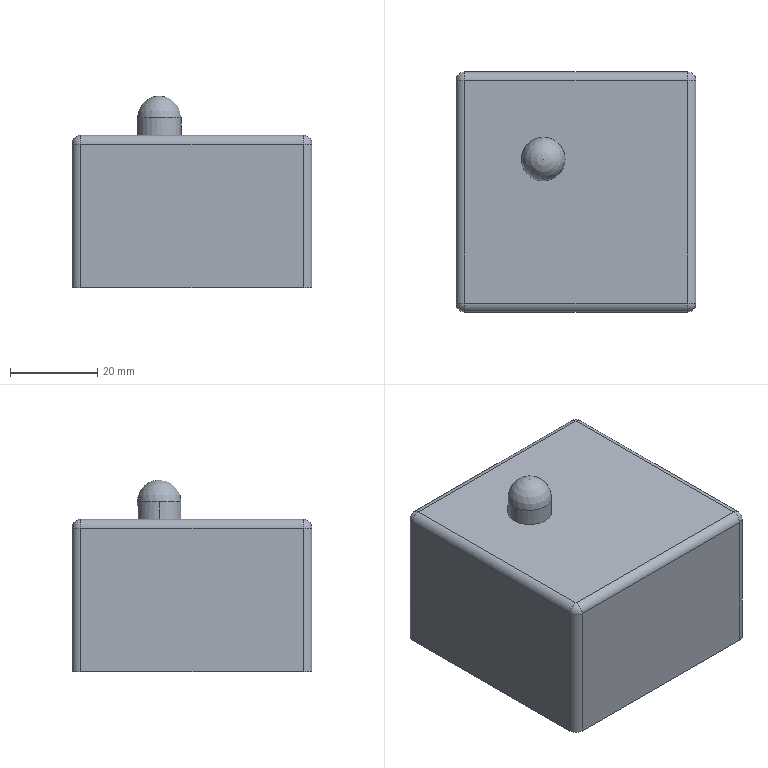Part | SolidWorks | features BaseBody 1 | 1 solid | 21 faces | box 55 x 55 x 44 mm | volume 106147 mm3 | cylinder 10 | plane 6 | sphere 5 | commonest cylinder face diameters 4 x8 10 x2
STEP:
#1=CARTESIAN_POINT('',(25.,-20.,39.));
#2=VERTEX_POINT('',#1);
#3=CARTESIAN_POINT('',(15.,-20.,39.));
#4=VERTEX_POINT('',#3);
#5=CARTESIAN_POINT('',(20.,-20.,39.));
#6=DIRECTION('',(0.,0.,1.));
#7=DIRECTION('',(1.,0.,0.));
#8=AXIS2_PLACEMENT_3D('',#5,#6,#7);
#9=CIRCLE('',#8,5.);
#10=EDGE_CURVE('',#2,#4,#9,.T.);
#11=ORIENTED_EDGE('',*,*,#10,.F.);
#12=CARTESIAN_POINT('',(25.,-20.,35.));
#13=VERTEX_POINT('',#12);
#14=CARTESIAN_POINT('',(25.,-20.,39.));
#15=DIRECTION('',(0.,0.,-1.));
#16=VECTOR('',#15,1000.);
#17=LINE('',#14,#16);
#18=EDGE_CURVE('',#2,#13,#17,.T.);
#19=ORIENTED_EDGE('',*,*,#18,.T.);
#20=CARTESIAN_POINT('',(15.,-20.,35.));
#21=VERTEX_POINT('',#20);
#22=CARTESIAN_POINT('',(20.,-20.,35.));
#23=DIRECTION('',(0.,0.,1.));
#24=DIRECTION('',(1.,0.,0.));
#25=AXIS2_PLACEMENT_3D('',#22,#23,#24);
#26=CIRCLE('',#25,5.);
#27=EDGE_CURVE('',#13,#21,#26,.T.);
#28=ORIENTED_EDGE('',*,*,#27,.T.);
#29=CARTESIAN_POINT('',(15.,-20.,39.));
#30=DIRECTION('',(0.,0.,-1.));
#31=VECTOR('',#30,1000.);
#32=LINE('',#29,#31);
#33=EDGE_CURVE('',#4,#21,#32,.T.);
#34=ORIENTED_EDGE('',*,*,#33,.F.);
#35=EDGE_LOOP('',(#11,#19,#28,#34));
#36=FACE_OUTER_BOUND('',#35,.T.);
#37=CARTESIAN_POINT('',(20.,-20.,39.));
#38=DIRECTION('',(0.,0.,-1.));
#39=DIRECTION('',(-1.,0.,0.));
#40=AXIS2_PLACEMENT_3D('',#37,#38,#39);
#41=CYLINDRICAL_SURFACE('',#40,5.);
#42=ADVANCED_FACE('',(#36),#41,.T.);
#43=CARTESIAN_POINT('',(0.,-2.,0.));
#44=VERTEX_POINT('',#43);
#45=CARTESIAN_POINT('',(0.,-53.,0.));
#46=VERTEX_POINT('',#45);
#47=CARTESIAN_POINT('',(0.,0.,0.));
#48=DIRECTION('',(0.,-1.,0.));
#49=VECTOR('',#48,1000.);
#50=LINE('',#47,#49);
#51=EDGE_CURVE('',#44,#46,#50,.T.);
#52=ORIENTED_EDGE('',*,*,#51,.T.);
#53=CARTESIAN_POINT('',(0.,-53.,33.));
#54=VERTEX_POINT('',#53);
#55=CARTESIAN_POINT('',(0.,-53.,35.));
#56=DIRECTION('',(0.,0.,1.));
#57=VECTOR('',#56,1000.);
#58=LINE('',#55,#57);
#59=EDGE_CURVE('',#46,#54,#58,.T.);
#60=ORIENTED_EDGE('',*,*,#59,.T.);
#61=CARTESIAN_POINT('',(0.,-2.,33.));
#62=VERTEX_POINT('',#61);
#63=CARTESIAN_POINT('',(0.,0.,33.));
#64=DIRECTION('',(0.,1.,0.));
#65=VECTOR('',#64,1000.);
#66=LINE('',#63,#65);
#67=EDGE_CURVE('',#54,#62,#66,.T.);
#68=ORIENTED_EDGE('',*,*,#67,.T.);
#69=CARTESIAN_POINT('',(0.,-2.,35.));
#70=DIRECTION('',(0.,0.,-1.));
#71=VECTOR('',#70,1000.);
#72=LINE('',#69,#71);
#73=EDGE_CURVE('',#62,#44,#72,.T.);
#74=ORIENTED_EDGE('',*,*,#73,.T.);
#75=EDGE_LOOP('',(#52,#60,#68,#74));
#76=FACE_OUTER_BOUND('',#75,.T.);
#77=CARTESIAN_POINT('',(0.,0.,35.));
#78=DIRECTION('',(1.,0.,0.));
#79=DIRECTION('',(0.,1.,0.));
#80=AXIS2_PLACEMENT_3D('',#77,#78,#79);
#81=PLANE('',#80);
#82=ADVANCED_FACE('',(#76),#81,.F.);
#83=CARTESIAN_POINT('',(53.,-55.,33.));
#84=VERTEX_POINT('',#83);
#85=CARTESIAN_POINT('',(2.,-55.,33.));
#86=VERTEX_POINT('',#85);
#87=CARTESIAN_POINT('',(0.,-55.,33.));
#88=DIRECTION('',(-1.,0.,0.));
#89=VECTOR('',#88,1000.);
#90=LINE('',#87,#89);
#91=EDGE_CURVE('',#84,#86,#90,.T.);
#92=ORIENTED_EDGE('',*,*,#91,.T.);
#93=CARTESIAN_POINT('',(2.,-55.,0.));
#94=VERTEX_POINT('',#93);
#95=CARTESIAN_POINT('',(2.,-55.,35.));
#96=DIRECTION('',(0.,0.,-1.));
#97=VECTOR('',#96,1000.);
#98=LINE('',#95,#97);
#99=EDGE_CURVE('',#86,#94,#98,.T.);
#100=ORIENTED_EDGE('',*,*,#99,.T.);
#101=CARTESIAN_POINT('',(53.,-55.,0.));
#102=VERTEX_POINT('',#101);
#103=CARTESIAN_POINT('',(0.,-55.,0.));
#104=DIRECTION('',(1.,0.,0.));
#105=VECTOR('',#104,1000.);
#106=LINE('',#103,#105);
#107=EDGE_CURVE('',#94,#102,#106,.T.);
#108=ORIENTED_EDGE('',*,*,#107,.T.);
#109=CARTESIAN_POINT('',(53.,-55.,35.));
#110=DIRECTION('',(0.,0.,1.));
#111=VECTOR('',#110,1000.);
#112=LINE('',#109,#111);
#113=EDGE_CURVE('',#102,#84,#112,.T.);
#114=ORIENTED_EDGE('',*,*,#113,.T.);
#115=EDGE_LOOP('',(#92,#100,#108,#114));
#116=FACE_OUTER_BOUND('',#115,.T.);
#117=CARTESIAN_POINT('',(0.,-55.,35.));
#118=DIRECTION('',(0.,1.,0.));
#119=DIRECTION('',(0.,0.,1.));
#120=AXIS2_PLACEMENT_3D('',#117,#118,#119);
#121=PLANE('',#120);
#122=ADVANCED_FACE('',(#116),#121,.F.);
#123=CARTESIAN_POINT('',(55.,-53.,0.));
#124=VERTEX_POINT('',#123);
#125=CARTESIAN_POINT('',(55.,-2.,0.));
#126=VERTEX_POINT('',#125);
#127=CARTESIAN_POINT('',(55.,0.,0.));
#128=DIRECTION('',(0.,1.,0.));
#129=VECTOR('',#128,1000.);
#130=LINE('',#127,#129);
#131=EDGE_CURVE('',#124,#126,#130,.T.);
#132=ORIENTED_EDGE('',*,*,#131,.T.);
#133=CARTESIAN_POINT('',(55.,-2.,33.));
#134=VERTEX_POINT('',#133);
#135=CARTESIAN_POINT('',(55.,-2.,35.));
#136=DIRECTION('',(0.,0.,1.));
#137=VECTOR('',#136,1000.);
#138=LINE('',#135,#137);
#139=EDGE_CURVE('',#126,#134,#138,.T.);
#140=ORIENTED_EDGE('',*,*,#139,.T.);
#141=CARTESIAN_POINT('',(55.,-53.,33.));
#142=VERTEX_POINT('',#141);
#143=CARTESIAN_POINT('',(55.,-55.,33.));
#144=DIRECTION('',(0.,-1.,0.));
#145=VECTOR('',#144,1000.);
#146=LINE('',#143,#145);
#147=EDGE_CURVE('',#134,#142,#146,.T.);
#148=ORIENTED_EDGE('',*,*,#147,.T.);
#149=CARTESIAN_POINT('',(55.,-53.,35.));
#150=DIRECTION('',(0.,0.,-1.));
#151=VECTOR('',#150,1000.);
#152=LINE('',#149,#151);
#153=EDGE_CURVE('',#142,#124,#152,.T.);
#154=ORIENTED_EDGE('',*,*,#153,.T.);
#155=EDGE_LOOP('',(#132,#140,#148,#154));
#156=FACE_OUTER_BOUND('',#155,.T.);
#157=CARTESIAN_POINT('',(55.,0.,35.));
#158=DIRECTION('',(-1.,0.,0.));
#159=DIRECTION('',(0.,0.,1.));
#160=AXIS2_PLACEMENT_3D('',#157,#158,#159);
#161=PLANE('',#160);
#162=ADVANCED_FACE('',(#156),#161,.F.);
#163=CARTESIAN_POINT('',(53.,0.,0.));
#164=VERTEX_POINT('',#163);
#165=CARTESIAN_POINT('',(2.,0.,0.));
#166=VERTEX_POINT('',#165);
#167=CARTESIAN_POINT('',(0.,0.,0.));
#168=DIRECTION('',(-1.,0.,0.));
#169=VECTOR('',#168,1000.);
#170=LINE('',#167,#169);
#171=EDGE_CURVE('',#164,#166,#170,.T.);
#172=ORIENTED_EDGE('',*,*,#171,.T.);
#173=CARTESIAN_POINT('',(2.,0.,33.));
#174=VERTEX_POINT('',#173);
#175=CARTESIAN_POINT('',(2.,0.,35.));
#176=DIRECTION('',(0.,0.,1.));
#177=VECTOR('',#176,1000.);
#178=LINE('',#175,#177);
#179=EDGE_CURVE('',#166,#174,#178,.T.);
#180=ORIENTED_EDGE('',*,*,#179,.T.);
#181=CARTESIAN_POINT('',(53.,0.,33.));
#182=VERTEX_POINT('',#181);
#183=CARTESIAN_POINT('',(55.,0.,33.));
#184=DIRECTION('',(1.,0.,0.));
#185=VECTOR('',#184,1000.);
#186=LINE('',#183,#185);
#187=EDGE_CURVE('',#174,#182,#186,.T.);
#188=ORIENTED_EDGE('',*,*,#187,.T.);
#189=CARTESIAN_POINT('',(53.,0.,35.));
#190=DIRECTION('',(0.,0.,-1.));
#191=VECTOR('',#190,1000.);
#192=LINE('',#189,#191);
#193=EDGE_CURVE('',#182,#164,#192,.T.);
#194=ORIENTED_EDGE('',*,*,#193,.T.);
#195=EDGE_LOOP('',(#172,#180,#188,#194));
#196=FACE_OUTER_BOUND('',#195,.T.);
#197=CARTESIAN_POINT('',(0.,0.,35.));
#198=DIRECTION('',(0.,-1.,0.));
#199=DIRECTION('',(0.,0.,-1.));
#200=AXIS2_PLACEMENT_3D('',#197,#198,#199);
#201=PLANE('',#200);
#202=ADVANCED_FACE('',(#196),#201,.F.);
#203=CARTESIAN_POINT('',(53.,-53.,35.));
#204=VERTEX_POINT('',#203);
#205=CARTESIAN_POINT('',(53.,-2.,35.));
#206=VERTEX_POINT('',#205);
#207=CARTESIAN_POINT('',(53.,0.,35.));
#208=DIRECTION('',(0.,1.,0.));
#209=VECTOR('',#208,1000.);
#210=LINE('',#207,#209);
#211=EDGE_CURVE('',#204,#206,#210,.T.);
#212=ORIENTED_EDGE('',*,*,#211,.T.);
#213=CARTESIAN_POINT('',(2.,-2.,35.));
#214=VERTEX_POINT('',#213);
#215=CARTESIAN_POINT('',(0.,-2.,35.));
#216=DIRECTION('',(-1.,0.,0.));
#217=VECTOR('',#216,1000.);
#218=LINE('',#215,#217);
#219=EDGE_CURVE('',#206,#214,#218,.T.);
#220=ORIENTED_EDGE('',*,*,#219,.T.);
#221=CARTESIAN_POINT('',(2.,-53.,35.));
#222=VERTEX_POINT('',#221);
#223=CARTESIAN_POINT('',(2.,-55.,35.));
#224=DIRECTION('',(0.,-1.,0.));
#225=VECTOR('',#224,1000.);
#226=LINE('',#223,#225);
#227=EDGE_CURVE('',#214,#222,#226,.T.);
#228=ORIENTED_EDGE('',*,*,#227,.T.);
#229=CARTESIAN_POINT('',(55.,-53.,35.));
#230=DIRECTION('',(1.,0.,0.));
#231=VECTOR('',#230,1000.);
#232=LINE('',#229,#231);
#233=EDGE_CURVE('',#222,#204,#232,.T.);
#234=ORIENTED_EDGE('',*,*,#233,.T.);
#235=EDGE_LOOP('',(#212,#220,#228,#234));
#236=FACE_OUTER_BOUND('',#235,.T.);
#237=CARTESIAN_POINT('',(20.,-20.,35.));
#238=DIRECTION('',(0.,0.,1.));
#239=DIRECTION('',(1.,0.,0.));
#240=AXIS2_PLACEMENT_3D('',#237,#238,#239);
#241=CIRCLE('',#240,5.);
#242=EDGE_CURVE('',#21,#13,#241,.T.);
#243=ORIENTED_EDGE('',*,*,#242,.F.);
#244=ORIENTED_EDGE('',*,*,#27,.F.);
#245=EDGE_LOOP('',(#243,#244));
#246=FACE_BOUND('',#245,.T.);
#247=CARTESIAN_POINT('',(0.,0.,35.));
#248=DIRECTION('',(0.,0.,1.));
#249=DIRECTION('',(1.,0.,0.));
#250=AXIS2_PLACEMENT_3D('',#247,#248,#249);
#251=PLANE('',#250);
#252=ADVANCED_FACE('',(#236,#246),#251,.T.);
#253=ORIENTED_EDGE('',*,*,#107,.F.);
#254=CARTESIAN_POINT('',(2.,-53.,0.));
#255=DIRECTION('',(0.,0.,-1.));
#256=DIRECTION('',(1.,0.,0.));
#257=AXIS2_PLACEMENT_3D('',#254,#255,#256);
#258=CIRCLE('',#257,2.);
#259=EDGE_CURVE('',#94,#46,#258,.T.);
#260=ORIENTED_EDGE('',*,*,#259,.T.);
#261=ORIENTED_EDGE('',*,*,#51,.F.);
#262=CARTESIAN_POINT('',(2.,-2.,0.));
#263=DIRECTION('',(0.,0.,-1.));
#264=DIRECTION('',(1.,0.,0.));
#265=AXIS2_PLACEMENT_3D('',#262,#263,#264);
#266=CIRCLE('',#265,2.);
#267=EDGE_CURVE('',#44,#166,#266,.T.);
#268=ORIENTED_EDGE('',*,*,#267,.T.);
#269=ORIENTED_EDGE('',*,*,#171,.F.);
#270=CARTESIAN_POINT('',(53.,-2.,0.));
#271=DIRECTION('',(0.,0.,-1.));
#272=DIRECTION('',(1.,0.,0.));
#273=AXIS2_PLACEMENT_3D('',#270,#271,#272);
#274=CIRCLE('',#273,2.);
#275=EDGE_CURVE('',#164,#126,#274,.T.);
#276=ORIENTED_EDGE('',*,*,#275,.T.);
#277=ORIENTED_EDGE('',*,*,#131,.F.);
#278=CARTESIAN_POINT('',(53.,-53.,0.));
#279=DIRECTION('',(0.,0.,-1.));
#280=DIRECTION('',(1.,0.,0.));
#281=AXIS2_PLACEMENT_3D('',#278,#279,#280);
#282=CIRCLE('',#281,2.);
#283=EDGE_CURVE('',#124,#102,#282,.T.);
#284=ORIENTED_EDGE('',*,*,#283,.T.);
#285=EDGE_LOOP('',(#253,#260,#261,#268,#269,#276,#277,#284));
#286=FACE_OUTER_BOUND('',#285,.T.);
#287=CARTESIAN_POINT('',(0.,0.,0.));
#288=DIRECTION('',(0.,0.,1.));
#289=DIRECTION('',(1.,0.,0.));
#290=AXIS2_PLACEMENT_3D('',#287,#288,#289);
#291=PLANE('',#290);
#292=ADVANCED_FACE('',(#286),#291,.F.);
#293=ORIENTED_EDGE('',*,*,#18,.F.);
#294=CARTESIAN_POINT('',(20.,-20.,39.));
#295=DIRECTION('',(0.,0.,1.));
#296=DIRECTION('',(1.,0.,0.));
#297=AXIS2_PLACEMENT_3D('',#294,#295,#296);
#298=CIRCLE('',#297,5.);
#299=EDGE_CURVE('',#4,#2,#298,.T.);
#300=ORIENTED_EDGE('',*,*,#299,.F.);
#301=ORIENTED_EDGE('',*,*,#33,.T.);
#302=ORIENTED_EDGE('',*,*,#242,.T.);
#303=EDGE_LOOP('',(#293,#300,#301,#302));
#304=FACE_OUTER_BOUND('',#303,.T.);
#305=CARTESIAN_POINT('',(20.,-20.,39.));
#306=DIRECTION('',(0.,0.,-1.));
#307=DIRECTION('',(-1.,0.,0.));
#308=AXIS2_PLACEMENT_3D('',#305,#306,#307);
#309=CYLINDRICAL_SURFACE('',#308,5.);
#310=ADVANCED_FACE('',(#304),#309,.T.);
#311=ORIENTED_EDGE('',*,*,#299,.T.);
#312=ORIENTED_EDGE('',*,*,#10,.T.);
#313=EDGE_LOOP('',(#311,#312));
#314=FACE_OUTER_BOUND('',#313,.T.);
#315=CARTESIAN_POINT('',(20.,-20.,39.));
#316=DIRECTION('',(0.,0.,-1.));
#317=DIRECTION('',(0.,1.,0.));
#318=AXIS2_PLACEMENT_3D('',#315,#316,#317);
#319=SPHERICAL_SURFACE('',#318,5.);
#320=ADVANCED_FACE('',(#314),#319,.T.);
#321=CARTESIAN_POINT('',(53.,-2.,33.));
#322=DIRECTION('',(0.,0.,1.));
#323=DIRECTION('',(1.,0.,0.));
#324=AXIS2_PLACEMENT_3D('',#321,#322,#323);
#325=CIRCLE('',#324,2.);
#326=EDGE_CURVE('',#134,#182,#325,.T.);
#327=ORIENTED_EDGE('',*,*,#326,.F.);
#328=ORIENTED_EDGE('',*,*,#139,.F.);
#329=ORIENTED_EDGE('',*,*,#275,.F.);
#330=ORIENTED_EDGE('',*,*,#193,.F.);
#331=EDGE_LOOP('',(#327,#328,#329,#330));
#332=FACE_OUTER_BOUND('',#331,.T.);
#333=CARTESIAN_POINT('',(53.,-2.,35.));
#334=DIRECTION('',(0.,0.,-1.));
#335=DIRECTION('',(-1.,0.,0.));
#336=AXIS2_PLACEMENT_3D('',#333,#334,#335);
#337=CYLINDRICAL_SURFACE('',#336,2.);
#338=ADVANCED_FACE('',(#332),#337,.T.);
#339=CARTESIAN_POINT('',(53.,-2.,33.));
#340=DIRECTION('',(0.,-1.,0.));
#341=DIRECTION('',(0.,0.,1.));
#342=AXIS2_PLACEMENT_3D('',#339,#340,#341);
#343=CIRCLE('',#342,2.);
#344=EDGE_CURVE('',#134,#206,#343,.T.);
#345=ORIENTED_EDGE('',*,*,#344,.F.);
#346=ORIENTED_EDGE('',*,*,#326,.T.);
#347=CARTESIAN_POINT('',(53.,-2.,33.));
#348=DIRECTION('',(-1.,0.,0.));
#349=DIRECTION('',(0.,0.,-1.));
#350=AXIS2_PLACEMENT_3D('',#347,#348,#349);
#351=CIRCLE('',#350,2.);
#352=EDGE_CURVE('',#206,#182,#351,.T.);
#353=ORIENTED_EDGE('',*,*,#352,.F.);
#354=EDGE_LOOP('',(#345,#346,#353));
#355=FACE_OUTER_BOUND('',#354,.T.);
#356=CARTESIAN_POINT('',(53.,-2.,33.));
#357=DIRECTION('',(0.,1.,0.));
#358=DIRECTION('',(1.,0.,0.));
#359=AXIS2_PLACEMENT_3D('',#356,#357,#358);
#360=SPHERICAL_SURFACE('',#359,2.);
#361=ADVANCED_FACE('',(#355),#360,.T.);
#362=ORIENTED_EDGE('',*,*,#267,.F.);
#363=ORIENTED_EDGE('',*,*,#73,.F.);
#364=CARTESIAN_POINT('',(2.,-2.,33.));
#365=DIRECTION('',(0.,0.,1.));
#366=DIRECTION('',(1.,0.,0.));
#367=AXIS2_PLACEMENT_3D('',#364,#365,#366);
#368=CIRCLE('',#367,2.);
#369=EDGE_CURVE('',#174,#62,#368,.T.);
#370=ORIENTED_EDGE('',*,*,#369,.F.);
#371=ORIENTED_EDGE('',*,*,#179,.F.);
#372=EDGE_LOOP('',(#362,#363,#370,#371));
#373=FACE_OUTER_BOUND('',#372,.T.);
#374=CARTESIAN_POINT('',(2.,-2.,35.));
#375=DIRECTION('',(0.,0.,-1.));
#376=DIRECTION('',(-1.,0.,0.));
#377=AXIS2_PLACEMENT_3D('',#374,#375,#376);
#378=CYLINDRICAL_SURFACE('',#377,2.);
#379=ADVANCED_FACE('',(#373),#378,.T.);
#380=ORIENTED_EDGE('',*,*,#352,.T.);
#381=ORIENTED_EDGE('',*,*,#187,.F.);
#382=CARTESIAN_POINT('',(2.,-2.,33.));
#383=DIRECTION('',(-1.,0.,0.));
#384=DIRECTION('',(0.,0.,1.));
#385=AXIS2_PLACEMENT_3D('',#382,#383,#384);
#386=CIRCLE('',#385,2.);
#387=EDGE_CURVE('',#214,#174,#386,.T.);
#388=ORIENTED_EDGE('',*,*,#387,.F.);
#389=ORIENTED_EDGE('',*,*,#219,.F.);
#390=EDGE_LOOP('',(#380,#381,#388,#389));
#391=FACE_OUTER_BOUND('',#390,.T.);
#392=CARTESIAN_POINT('',(0.,-2.,33.));
#393=DIRECTION('',(1.,0.,0.));
#394=DIRECTION('',(0.,0.,-1.));
#395=AXIS2_PLACEMENT_3D('',#392,#393,#394);
#396=CYLINDRICAL_SURFACE('',#395,2.);
#397=ADVANCED_FACE('',(#391),#396,.T.);
#398=ORIENTED_EDGE('',*,*,#344,.T.);
#399=ORIENTED_EDGE('',*,*,#211,.F.);
#400=CARTESIAN_POINT('',(53.,-53.,33.));
#401=DIRECTION('',(0.,-1.,0.));
#402=DIRECTION('',(0.,0.,-1.));
#403=AXIS2_PLACEMENT_3D('',#400,#401,#402);
#404=CIRCLE('',#403,2.);
#405=EDGE_CURVE('',#142,#204,#404,.T.);
#406=ORIENTED_EDGE('',*,*,#405,.F.);
#407=ORIENTED_EDGE('',*,*,#147,.F.);
#408=EDGE_LOOP('',(#398,#399,#406,#407));
#409=FACE_OUTER_BOUND('',#408,.T.);
#410=CARTESIAN_POINT('',(53.,0.,33.));
#411=DIRECTION('',(0.,-1.,0.));
#412=DIRECTION('',(0.,0.,-1.));
#413=AXIS2_PLACEMENT_3D('',#410,#411,#412);
#414=CYLINDRICAL_SURFACE('',#413,2.);
#415=ADVANCED_FACE('',(#409),#414,.T.);
#416=ORIENTED_EDGE('',*,*,#283,.F.);
#417=ORIENTED_EDGE('',*,*,#153,.F.);
#418=CARTESIAN_POINT('',(53.,-53.,33.));
#419=DIRECTION('',(0.,0.,1.));
#420=DIRECTION('',(1.,0.,0.));
#421=AXIS2_PLACEMENT_3D('',#418,#419,#420);
#422=CIRCLE('',#421,2.);
#423=EDGE_CURVE('',#84,#142,#422,.T.);
#424=ORIENTED_EDGE('',*,*,#423,.F.);
#425=ORIENTED_EDGE('',*,*,#113,.F.);
#426=EDGE_LOOP('',(#416,#417,#424,#425));
#427=FACE_OUTER_BOUND('',#426,.T.);
#428=CARTESIAN_POINT('',(53.,-53.,35.));
#429=DIRECTION('',(0.,0.,-1.));
#430=DIRECTION('',(-1.,0.,0.));
#431=AXIS2_PLACEMENT_3D('',#428,#429,#430);
#432=CYLINDRICAL_SURFACE('',#431,2.);
#433=ADVANCED_FACE('',(#427),#432,.T.);
#434=ORIENTED_EDGE('',*,*,#387,.T.);
#435=ORIENTED_EDGE('',*,*,#369,.T.);
#436=CARTESIAN_POINT('',(2.,-2.,33.));
#437=DIRECTION('',(0.,-1.,0.));
#438=DIRECTION('',(-1.,0.,0.));
#439=AXIS2_PLACEMENT_3D('',#436,#437,#438);
#440=CIRCLE('',#439,2.);
#441=EDGE_CURVE('',#214,#62,#440,.T.);
#442=ORIENTED_EDGE('',*,*,#441,.F.);
#443=EDGE_LOOP('',(#434,#435,#442));
#444=FACE_OUTER_BOUND('',#443,.T.);
#445=CARTESIAN_POINT('',(2.,-2.,33.));
#446=DIRECTION('',(0.,1.,0.));
#447=DIRECTION('',(1.,0.,0.));
#448=AXIS2_PLACEMENT_3D('',#445,#446,#447);
#449=SPHERICAL_SURFACE('',#448,2.);
#450=ADVANCED_FACE('',(#444),#449,.T.);
#451=ORIENTED_EDGE('',*,*,#423,.T.);
#452=ORIENTED_EDGE('',*,*,#405,.T.);
#453=CARTESIAN_POINT('',(53.,-53.,33.));
#454=DIRECTION('',(-1.,0.,0.));
#455=DIRECTION('',(0.,0.,-1.));
#456=AXIS2_PLACEMENT_3D('',#453,#454,#455);
#457=CIRCLE('',#456,2.);
#458=EDGE_CURVE('',#84,#204,#457,.T.);
#459=ORIENTED_EDGE('',*,*,#458,.F.);
#460=EDGE_LOOP('',(#451,#452,#459));
#461=FACE_OUTER_BOUND('',#460,.T.);
#462=CARTESIAN_POINT('',(53.,-53.,33.));
#463=DIRECTION('',(0.,1.,0.));
#464=DIRECTION('',(1.,0.,0.));
#465=AXIS2_PLACEMENT_3D('',#462,#463,#464);
#466=SPHERICAL_SURFACE('',#465,2.);
#467=ADVANCED_FACE('',(#461),#466,.T.);
#468=ORIENTED_EDGE('',*,*,#441,.T.);
#469=ORIENTED_EDGE('',*,*,#67,.F.);
#470=CARTESIAN_POINT('',(2.,-53.,33.));
#471=DIRECTION('',(0.,-1.,0.));
#472=DIRECTION('',(0.,0.,-1.));
#473=AXIS2_PLACEMENT_3D('',#470,#471,#472);
#474=CIRCLE('',#473,2.);
#475=EDGE_CURVE('',#222,#54,#474,.T.);
#476=ORIENTED_EDGE('',*,*,#475,.F.);
#477=ORIENTED_EDGE('',*,*,#227,.F.);
#478=EDGE_LOOP('',(#468,#469,#476,#477));
#479=FACE_OUTER_BOUND('',#478,.T.);
#480=CARTESIAN_POINT('',(2.,0.,33.));
#481=DIRECTION('',(0.,1.,0.));
#482=DIRECTION('',(-1.,0.,0.));
#483=AXIS2_PLACEMENT_3D('',#480,#481,#482);
#484=CYLINDRICAL_SURFACE('',#483,2.);
#485=ADVANCED_FACE('',(#479),#484,.T.);
#486=ORIENTED_EDGE('',*,*,#458,.T.);
#487=ORIENTED_EDGE('',*,*,#233,.F.);
#488=CARTESIAN_POINT('',(2.,-53.,33.));
#489=DIRECTION('',(-1.,0.,0.));
#490=DIRECTION('',(0.,0.,1.));
#491=AXIS2_PLACEMENT_3D('',#488,#489,#490);
#492=CIRCLE('',#491,2.);
#493=EDGE_CURVE('',#86,#222,#492,.T.);
#494=ORIENTED_EDGE('',*,*,#493,.F.);
#495=ORIENTED_EDGE('',*,*,#91,.F.);
#496=EDGE_LOOP('',(#486,#487,#494,#495));
#497=FACE_OUTER_BOUND('',#496,.T.);
#498=CARTESIAN_POINT('',(0.,-53.,33.));
#499=DIRECTION('',(-1.,0.,0.));
#500=DIRECTION('',(0.,0.,1.));
#501=AXIS2_PLACEMENT_3D('',#498,#499,#500);
#502=CYLINDRICAL_SURFACE('',#501,2.);
#503=ADVANCED_FACE('',(#497),#502,.T.);
#504=ORIENTED_EDGE('',*,*,#493,.T.);
#505=ORIENTED_EDGE('',*,*,#475,.T.);
#506=CARTESIAN_POINT('',(2.,-53.,33.));
#507=DIRECTION('',(0.,0.,-1.));
#508=DIRECTION('',(1.,0.,0.));
#509=AXIS2_PLACEMENT_3D('',#506,#507,#508);
#510=CIRCLE('',#509,2.);
#511=EDGE_CURVE('',#86,#54,#510,.T.);
#512=ORIENTED_EDGE('',*,*,#511,.F.);
#513=EDGE_LOOP('',(#504,#505,#512));
#514=FACE_OUTER_BOUND('',#513,.T.);
#515=CARTESIAN_POINT('',(2.,-53.,33.));
#516=DIRECTION('',(0.,1.,0.));
#517=DIRECTION('',(1.,0.,0.));
#518=AXIS2_PLACEMENT_3D('',#515,#516,#517);
#519=SPHERICAL_SURFACE('',#518,2.);
#520=ADVANCED_FACE('',(#514),#519,.T.);
#521=ORIENTED_EDGE('',*,*,#511,.T.);
#522=ORIENTED_EDGE('',*,*,#59,.F.);
#523=ORIENTED_EDGE('',*,*,#259,.F.);
#524=ORIENTED_EDGE('',*,*,#99,.F.);
#525=EDGE_LOOP('',(#521,#522,#523,#524));
#526=FACE_OUTER_BOUND('',#525,.T.);
#527=CARTESIAN_POINT('',(2.,-53.,35.));
#528=DIRECTION('',(0.,0.,-1.));
#529=DIRECTION('',(-1.,0.,0.));
#530=AXIS2_PLACEMENT_3D('',#527,#528,#529);
#531=CYLINDRICAL_SURFACE('',#530,2.);
#532=ADVANCED_FACE('',(#526),#531,.T.);
#533=CLOSED_SHELL('',(#42,#82,#122,#162,#202,#252,#292,#310,#320,#338,#361,#379,#397,#415,#433,#450,#467,#485,#503,#520,#532));
#534=MANIFOLD_SOLID_BREP('',#533);
#535=CARTESIAN_POINT('',(0.,0.,0.));
#536=DIRECTION('',(0.,0.,1.));
#537=DIRECTION('',(1.,0.,0.));
#538=AXIS2_PLACEMENT_3D('',#535,#536,#537);
#539=(LENGTH_UNIT()NAMED_UNIT(*)SI_UNIT(.MILLI.,.METRE.));
#540=UNCERTAINTY_MEASURE_WITH_UNIT(LENGTH_MEASURE(0.00001),#539,'','');
#541=(NAMED_UNIT(*)PLANE_ANGLE_UNIT()SI_UNIT($,.RADIAN.));
#542=(NAMED_UNIT(*)SI_UNIT($,.STERADIAN.)SOLID_ANGLE_UNIT());
#543=(GEOMETRIC_REPRESENTATION_CONTEXT(3)GLOBAL_UNCERTAINTY_ASSIGNED_CONTEXT((#540))GLOBAL_UNIT_ASSIGNED_CONTEXT((#539,#541,#542))REPRESENTATION_CONTEXT('',''));
#544=ADVANCED_BREP_SHAPE_REPRESENTATION('',(#534,#538),#543);